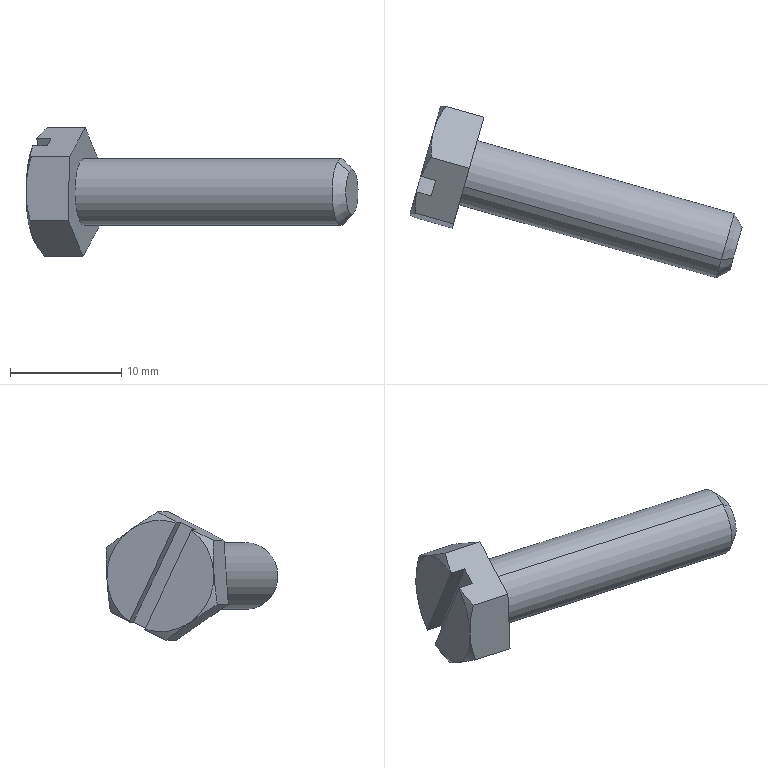Part | SolidWorks | features BaseBody 1 | 1 solid | 23 faces | box 29.808 x 15.418 x 11.521 mm | volume 1021 mm3 | plane 13 | cone 8 | cylinder 2 | commonest cylinder face diameters 6 x2
STEP:
#1=CARTESIAN_POINT('',(393.299,90.116,55.705));
#2=VERTEX_POINT('',#1);
#3=CARTESIAN_POINT('',(392.816,88.42,59.295));
#4=VERTEX_POINT('',#3);
#5=CARTESIAN_POINT('',(393.058,89.268,57.5));
#6=DIRECTION('',(0.9618,-0.2738,0.));
#7=DIRECTION('',(0.1207,0.424,-0.8976));
#8=AXIS2_PLACEMENT_3D('',#5,#6,#7);
#9=CIRCLE('',#8,2.);
#10=EDGE_CURVE('',#2,#4,#9,.T.);
#11=ORIENTED_EDGE('',*,*,#10,.F.);
#12=CARTESIAN_POINT('',(392.458,90.814,54.807));
#13=VERTEX_POINT('',#12);
#14=CARTESIAN_POINT('',(393.299,90.116,55.705));
#15=DIRECTION('',(-0.5947,0.4934,-0.6347));
#16=VECTOR('',#15,1000.);
#17=LINE('',#14,#16);
#18=EDGE_CURVE('',#2,#13,#17,.T.);
#19=ORIENTED_EDGE('',*,*,#18,.T.);
#20=CARTESIAN_POINT('',(391.734,88.27,60.193));
#21=VERTEX_POINT('',#20);
#22=CARTESIAN_POINT('',(392.096,89.542,57.5));
#23=DIRECTION('',(-0.9618,0.2738,0.));
#24=DIRECTION('',(0.1207,0.424,-0.8976));
#25=AXIS2_PLACEMENT_3D('',#22,#23,#24);
#26=CIRCLE('',#25,3.);
#27=EDGE_CURVE('',#21,#13,#26,.T.);
#28=ORIENTED_EDGE('',*,*,#27,.F.);
#29=CARTESIAN_POINT('',(392.816,88.42,59.295));
#30=DIRECTION('',(-0.7654,-0.1062,0.6347));
#31=VECTOR('',#30,1000.);
#32=LINE('',#29,#31);
#33=EDGE_CURVE('',#4,#21,#32,.T.);
#34=ORIENTED_EDGE('',*,*,#33,.F.);
#35=EDGE_LOOP('',(#11,#19,#28,#34));
#36=FACE_OUTER_BOUND('',#35,.T.);
#37=CARTESIAN_POINT('',(393.058,89.268,57.5));
#38=DIRECTION('',(-0.9618,0.2738,0.));
#39=DIRECTION('',(-0.1207,-0.424,0.8976));
#40=AXIS2_PLACEMENT_3D('',#37,#38,#39);
#41=CONICAL_SURFACE('',#40,2.,0.7854);
#42=ADVANCED_FACE('',(#36),#41,.T.);
#43=ORIENTED_EDGE('',*,*,#27,.T.);
#44=CARTESIAN_POINT('',(369.375,97.385,54.807));
#45=VERTEX_POINT('',#44);
#46=CARTESIAN_POINT('',(393.42,90.54,54.807));
#47=DIRECTION('',(-0.9618,0.2738,0.));
#48=VECTOR('',#47,1000.);
#49=LINE('',#46,#48);
#50=EDGE_CURVE('',#13,#45,#49,.T.);
#51=ORIENTED_EDGE('',*,*,#50,.T.);
#52=CARTESIAN_POINT('',(368.651,94.841,60.193));
#53=VERTEX_POINT('',#52);
#54=CARTESIAN_POINT('',(369.013,96.113,57.5));
#55=DIRECTION('',(0.9618,-0.2738,0.));
#56=DIRECTION('',(0.1207,0.424,-0.8976));
#57=AXIS2_PLACEMENT_3D('',#54,#55,#56);
#58=CIRCLE('',#57,3.);
#59=EDGE_CURVE('',#45,#53,#58,.T.);
#60=ORIENTED_EDGE('',*,*,#59,.T.);
#61=CARTESIAN_POINT('',(392.696,87.996,60.193));
#62=DIRECTION('',(-0.9618,0.2738,0.));
#63=VECTOR('',#62,1000.);
#64=LINE('',#61,#63);
#65=EDGE_CURVE('',#21,#53,#64,.T.);
#66=ORIENTED_EDGE('',*,*,#65,.F.);
#67=EDGE_LOOP('',(#43,#51,#60,#66));
#68=FACE_OUTER_BOUND('',#67,.T.);
#69=CARTESIAN_POINT('',(393.058,89.268,57.5));
#70=DIRECTION('',(-0.9618,0.2738,0.));
#71=DIRECTION('',(-0.1207,-0.424,0.8976));
#72=AXIS2_PLACEMENT_3D('',#69,#70,#71);
#73=CYLINDRICAL_SURFACE('',#72,3.);
#74=ADVANCED_FACE('',(#68),#73,.T.);
#75=CARTESIAN_POINT('',(370.432,101.097,60.045));
#76=VERTEX_POINT('',#75);
#77=CARTESIAN_POINT('',(369.119,96.485,63.261));
#78=VERTEX_POINT('',#77);
#79=CARTESIAN_POINT('',(369.119,96.485,63.261));
#80=DIRECTION('',(-0.2274,-0.7988,0.5569));
#81=VECTOR('',#80,1000.);
#82=LINE('',#79,#81);
#83=EDGE_CURVE('',#76,#78,#82,.T.);
#84=ORIENTED_EDGE('',*,*,#83,.T.);
#85=CARTESIAN_POINT('',(367.7,91.501,60.715));
#86=VERTEX_POINT('',#85);
#87=CARTESIAN_POINT('',(367.7,91.501,60.715));
#88=DIRECTION('',(-0.2457,-0.8633,-0.4409));
#89=VECTOR('',#88,1000.);
#90=LINE('',#87,#89);
#91=EDGE_CURVE('',#78,#86,#90,.T.);
#92=ORIENTED_EDGE('',*,*,#91,.T.);
#93=CARTESIAN_POINT('',(367.594,91.129,54.955));
#94=VERTEX_POINT('',#93);
#95=CARTESIAN_POINT('',(367.7,91.501,60.715));
#96=DIRECTION('',(-0.01834,-0.06444,-0.9978));
#97=VECTOR('',#96,1000.);
#98=LINE('',#95,#97);
#99=EDGE_CURVE('',#86,#94,#98,.T.);
#100=ORIENTED_EDGE('',*,*,#99,.T.);
#101=CARTESIAN_POINT('',(368.907,95.741,51.739));
#102=VERTEX_POINT('',#101);
#103=CARTESIAN_POINT('',(368.907,95.741,51.739));
#104=DIRECTION('',(0.2274,0.7988,-0.5569));
#105=VECTOR('',#104,1000.);
#106=LINE('',#103,#105);
#107=EDGE_CURVE('',#94,#102,#106,.T.);
#108=ORIENTED_EDGE('',*,*,#107,.T.);
#109=CARTESIAN_POINT('',(370.326,100.725,54.285));
#110=VERTEX_POINT('',#109);
#111=CARTESIAN_POINT('',(368.907,95.741,51.739));
#112=DIRECTION('',(0.2457,0.8633,0.4409));
#113=VECTOR('',#112,1000.);
#114=LINE('',#111,#113);
#115=EDGE_CURVE('',#102,#110,#114,.T.);
#116=ORIENTED_EDGE('',*,*,#115,.T.);
#117=CARTESIAN_POINT('',(370.326,100.725,54.285));
#118=DIRECTION('',(0.01834,0.06444,0.9978));
#119=VECTOR('',#118,1000.);
#120=LINE('',#117,#119);
#121=EDGE_CURVE('',#110,#76,#120,.T.);
#122=ORIENTED_EDGE('',*,*,#121,.T.);
#123=EDGE_LOOP('',(#84,#92,#100,#108,#116,#122));
#124=FACE_OUTER_BOUND('',#123,.T.);
#125=CARTESIAN_POINT('',(369.013,96.113,57.5));
#126=DIRECTION('',(0.9618,-0.2738,0.));
#127=DIRECTION('',(0.1207,0.424,-0.8976));
#128=AXIS2_PLACEMENT_3D('',#125,#126,#127);
#129=CIRCLE('',#128,3.);
#130=EDGE_CURVE('',#53,#45,#129,.T.);
#131=ORIENTED_EDGE('',*,*,#130,.F.);
#132=ORIENTED_EDGE('',*,*,#59,.F.);
#133=EDGE_LOOP('',(#131,#132));
#134=FACE_BOUND('',#133,.T.);
#135=CARTESIAN_POINT('',(369.119,96.485,63.261));
#136=DIRECTION('',(0.9618,-0.2738,0.));
#137=DIRECTION('',(0.1207,0.424,-0.8976));
#138=AXIS2_PLACEMENT_3D('',#135,#136,#137);
#139=PLANE('',#138);
#140=ADVANCED_FACE('',(#124,#134),#139,.T.);
#141=CARTESIAN_POINT('',(363.8,92.41,57.835));
#142=VERTEX_POINT('',#141);
#143=CARTESIAN_POINT('',(364.374,94.424,61.577));
#144=VERTEX_POINT('',#143);
#145=CARTESIAN_POINT('',(365.166,97.208,57.5));
#146=DIRECTION('',(-0.9618,0.2738,0.));
#147=DIRECTION('',(-0.1207,-0.424,0.8976));
#148=AXIS2_PLACEMENT_3D('',#145,#146,#147);
#149=CIRCLE('',#148,5.);
#150=EDGE_CURVE('',#142,#144,#149,.T.);
#151=ORIENTED_EDGE('',*,*,#150,.T.);
#152=CARTESIAN_POINT('',(365.565,98.61,52.717));
#153=VERTEX_POINT('',#152);
#154=CARTESIAN_POINT('',(365.573,98.637,52.659));
#155=DIRECTION('',(-0.1207,-0.424,0.8976));
#156=VECTOR('',#155,1000.);
#157=LINE('',#154,#156);
#158=EDGE_CURVE('',#153,#144,#157,.T.);
#159=ORIENTED_EDGE('',*,*,#158,.F.);
#160=CARTESIAN_POINT('',(364.404,94.53,53.347));
#161=VERTEX_POINT('',#160);
#162=CARTESIAN_POINT('',(365.166,97.208,57.5));
#163=DIRECTION('',(-0.9618,0.2738,0.));
#164=DIRECTION('',(-0.1207,-0.424,0.8976));
#165=AXIS2_PLACEMENT_3D('',#162,#163,#164);
#166=CIRCLE('',#165,5.);
#167=EDGE_CURVE('',#153,#161,#166,.T.);
#168=ORIENTED_EDGE('',*,*,#167,.T.);
#169=CARTESIAN_POINT('',(365.166,97.208,57.5));
#170=DIRECTION('',(-0.9618,0.2738,0.));
#171=DIRECTION('',(-0.1207,-0.424,0.8976));
#172=AXIS2_PLACEMENT_3D('',#169,#170,#171);
#173=CIRCLE('',#172,5.);
#174=EDGE_CURVE('',#161,#142,#173,.T.);
#175=ORIENTED_EDGE('',*,*,#174,.T.);
#176=EDGE_LOOP('',(#151,#159,#168,#175));
#177=FACE_OUTER_BOUND('',#176,.T.);
#178=CARTESIAN_POINT('',(365.272,97.58,63.261));
#179=DIRECTION('',(0.9618,-0.2738,0.));
#180=DIRECTION('',(0.1207,0.424,-0.8976));
#181=AXIS2_PLACEMENT_3D('',#178,#179,#180);
#182=PLANE('',#181);
#183=ADVANCED_FACE('',(#177),#182,.F.);
#184=CARTESIAN_POINT('',(365.701,97.458,63.261));
#185=VERTEX_POINT('',#184);
#186=CARTESIAN_POINT('',(365.928,99.886,61.653));
#187=VERTEX_POINT('',#186);
#188=CARTESIAN_POINT('',(365.701,97.458,63.261));
#189=CARTESIAN_POINT('',(365.654,98.287,62.735));
#190=CARTESIAN_POINT('',(365.705,99.1,62.201));
#191=CARTESIAN_POINT('',(365.928,99.886,61.653));
#192=B_SPLINE_CURVE_WITH_KNOTS('',3,(#188,#189,#190,#191),.UNSPECIFIED.,.F.,.F.,(4,4),(0.000000238,0.002921),.UNSPECIFIED.);
#193=EDGE_CURVE('',#185,#187,#192,.T.);
#194=ORIENTED_EDGE('',*,*,#193,.F.);
#195=CARTESIAN_POINT('',(369.119,96.485,63.261));
#196=DIRECTION('',(-0.9618,0.2738,0.));
#197=VECTOR('',#196,1000.);
#198=LINE('',#195,#197);
#199=EDGE_CURVE('',#78,#185,#198,.T.);
#200=ORIENTED_EDGE('',*,*,#199,.F.);
#201=ORIENTED_EDGE('',*,*,#83,.F.);
#202=CARTESIAN_POINT('',(367.014,102.07,60.045));
#203=VERTEX_POINT('',#202);
#204=CARTESIAN_POINT('',(370.432,101.097,60.045));
#205=DIRECTION('',(-0.9618,0.2738,0.));
#206=VECTOR('',#205,1000.);
#207=LINE('',#204,#206);
#208=EDGE_CURVE('',#76,#203,#207,.T.);
#209=ORIENTED_EDGE('',*,*,#208,.T.);
#210=CARTESIAN_POINT('',(365.928,99.886,61.653));
#211=CARTESIAN_POINT('',(365.984,100.082,61.516));
#212=CARTESIAN_POINT('',(366.05,100.275,61.379));
#213=CARTESIAN_POINT('',(366.2,100.653,61.108));
#214=CARTESIAN_POINT('',(366.284,100.838,60.974));
#215=CARTESIAN_POINT('',(366.56,101.382,60.572));
#216=CARTESIAN_POINT('',(366.776,101.731,60.308));
#217=CARTESIAN_POINT('',(367.014,102.07,60.045));
#218=B_SPLINE_CURVE_WITH_KNOTS('',3,(#210,#211,#212,#213,#214,#215,#216,#217),.UNSPECIFIED.,.F.,.F.,(4,2,2,4),(0.002921,0.003649,0.004376,0.005831),.UNSPECIFIED.);
#219=EDGE_CURVE('',#187,#203,#218,.T.);
#220=ORIENTED_EDGE('',*,*,#219,.F.);
#221=EDGE_LOOP('',(#194,#200,#201,#209,#220));
#222=FACE_OUTER_BOUND('',#221,.T.);
#223=CARTESIAN_POINT('',(369.119,96.485,63.261));
#224=DIRECTION('',(-0.1525,-0.5356,-0.8306));
#225=DIRECTION('',(0.2274,0.7988,-0.5569));
#226=AXIS2_PLACEMENT_3D('',#223,#224,#225);
#227=PLANE('',#226);
#228=ADVANCED_FACE('',(#222),#227,.F.);
#229=CARTESIAN_POINT('',(364.283,92.473,60.715));
#230=VERTEX_POINT('',#229);
#231=CARTESIAN_POINT('',(364.401,94.387,61.635));
#232=VERTEX_POINT('',#231);
#233=CARTESIAN_POINT('',(364.283,92.473,60.715));
#234=CARTESIAN_POINT('',(364.272,92.795,60.866));
#235=CARTESIAN_POINT('',(364.273,93.119,61.019));
#236=CARTESIAN_POINT('',(364.31,93.758,61.326));
#237=CARTESIAN_POINT('',(364.346,94.075,61.48));
#238=CARTESIAN_POINT('',(364.401,94.387,61.635));
#239=B_SPLINE_CURVE_WITH_KNOTS('',3,(#233,#234,#235,#236,#237,#238),.UNSPECIFIED.,.F.,.F.,(4,2,4),(0.005386,0.006447,0.007508),.UNSPECIFIED.);
#240=EDGE_CURVE('',#230,#232,#239,.T.);
#241=ORIENTED_EDGE('',*,*,#240,.F.);
#242=CARTESIAN_POINT('',(367.7,91.501,60.715));
#243=DIRECTION('',(-0.9618,0.2738,0.));
#244=VECTOR('',#243,1000.);
#245=LINE('',#242,#244);
#246=EDGE_CURVE('',#86,#230,#245,.T.);
#247=ORIENTED_EDGE('',*,*,#246,.F.);
#248=ORIENTED_EDGE('',*,*,#91,.F.);
#249=ORIENTED_EDGE('',*,*,#199,.T.);
#250=CARTESIAN_POINT('',(364.794,95.768,62.341));
#251=VERTEX_POINT('',#250);
#252=CARTESIAN_POINT('',(364.794,95.768,62.341));
#253=CARTESIAN_POINT('',(365.032,96.367,62.655));
#254=CARTESIAN_POINT('',(365.345,96.924,62.961));
#255=CARTESIAN_POINT('',(365.701,97.458,63.261));
#256=B_SPLINE_CURVE_WITH_KNOTS('',3,(#252,#253,#254,#255),.UNSPECIFIED.,.F.,.F.,(4,4),(0.009104,0.01123),.UNSPECIFIED.);
#257=EDGE_CURVE('',#251,#185,#256,.T.);
#258=ORIENTED_EDGE('',*,*,#257,.F.);
#259=CARTESIAN_POINT('',(366.105,95.395,62.341));
#260=VERTEX_POINT('',#259);
#261=CARTESIAN_POINT('',(366.105,95.395,62.341));
#262=DIRECTION('',(-0.9618,0.2738,0.));
#263=VECTOR('',#262,1000.);
#264=LINE('',#261,#263);
#265=EDGE_CURVE('',#260,#251,#264,.T.);
#266=ORIENTED_EDGE('',*,*,#265,.F.);
#267=CARTESIAN_POINT('',(365.712,94.014,61.635));
#268=VERTEX_POINT('',#267);
#269=CARTESIAN_POINT('',(366.105,95.395,62.341));
#270=DIRECTION('',(0.2457,0.8633,0.4409));
#271=VECTOR('',#270,1000.);
#272=LINE('',#269,#271);
#273=EDGE_CURVE('',#268,#260,#272,.T.);
#274=ORIENTED_EDGE('',*,*,#273,.F.);
#275=CARTESIAN_POINT('',(365.712,94.014,61.635));
#276=DIRECTION('',(-0.9618,0.2738,0.));
#277=VECTOR('',#276,1000.);
#278=LINE('',#275,#277);
#279=EDGE_CURVE('',#268,#232,#278,.T.);
#280=ORIENTED_EDGE('',*,*,#279,.T.);
#281=EDGE_LOOP('',(#241,#247,#248,#249,#258,#266,#274,#280));
#282=FACE_OUTER_BOUND('',#281,.T.);
#283=CARTESIAN_POINT('',(367.7,91.501,60.715));
#284=DIRECTION('',(0.1207,0.424,-0.8976));
#285=DIRECTION('',(0.2457,0.8633,0.4409));
#286=AXIS2_PLACEMENT_3D('',#283,#284,#285);
#287=PLANE('',#286);
#288=ADVANCED_FACE('',(#282),#287,.F.);
#289=CARTESIAN_POINT('',(364.177,92.101,54.955));
#290=VERTEX_POINT('',#289);
#291=CARTESIAN_POINT('',(364.177,92.101,54.955));
#292=CARTESIAN_POINT('',(363.932,92.237,55.897));
#293=CARTESIAN_POINT('',(363.782,92.346,56.854));
#294=CARTESIAN_POINT('',(363.8,92.41,57.835));
#295=B_SPLINE_CURVE_WITH_KNOTS('',3,(#291,#292,#293,#294),.UNSPECIFIED.,.F.,.F.,(4,4),(0.000000238,0.002921),.UNSPECIFIED.);
#296=EDGE_CURVE('',#290,#142,#295,.T.);
#297=ORIENTED_EDGE('',*,*,#296,.F.);
#298=CARTESIAN_POINT('',(367.594,91.129,54.955));
#299=DIRECTION('',(-0.9618,0.2738,0.));
#300=VECTOR('',#299,1000.);
#301=LINE('',#298,#300);
#302=EDGE_CURVE('',#94,#290,#301,.T.);
#303=ORIENTED_EDGE('',*,*,#302,.F.);
#304=ORIENTED_EDGE('',*,*,#99,.F.);
#305=ORIENTED_EDGE('',*,*,#246,.T.);
#306=CARTESIAN_POINT('',(363.8,92.41,57.835));
#307=CARTESIAN_POINT('',(363.805,92.425,58.079));
#308=CARTESIAN_POINT('',(363.819,92.438,58.325));
#309=CARTESIAN_POINT('',(363.867,92.459,58.811));
#310=CARTESIAN_POINT('',(363.901,92.466,59.052));
#311=CARTESIAN_POINT('',(364.026,92.48,59.771));
#312=CARTESIAN_POINT('',(364.143,92.48,60.245));
#313=CARTESIAN_POINT('',(364.283,92.473,60.715));
#314=B_SPLINE_CURVE_WITH_KNOTS('',3,(#306,#307,#308,#309,#310,#311,#312,#313),.UNSPECIFIED.,.F.,.F.,(4,2,2,4),(0.002921,0.003649,0.004376,0.005831),.UNSPECIFIED.);
#315=EDGE_CURVE('',#142,#230,#314,.T.);
#316=ORIENTED_EDGE('',*,*,#315,.F.);
#317=EDGE_LOOP('',(#297,#303,#304,#305,#316));
#318=FACE_OUTER_BOUND('',#317,.T.);
#319=CARTESIAN_POINT('',(367.7,91.501,60.715));
#320=DIRECTION('',(0.2732,0.9596,-0.067));
#321=DIRECTION('',(0.01834,0.06444,0.9978));
#322=AXIS2_PLACEMENT_3D('',#319,#320,#321);
#323=PLANE('',#322);
#324=ADVANCED_FACE('',(#318),#323,.F.);
#325=CARTESIAN_POINT('',(365.489,96.714,51.739));
#326=VERTEX_POINT('',#325);
#327=CARTESIAN_POINT('',(365.489,96.714,51.739));
#328=CARTESIAN_POINT('',(365.012,96.034,52.265));
#329=CARTESIAN_POINT('',(364.627,95.315,52.799));
#330=CARTESIAN_POINT('',(364.404,94.53,53.347));
#331=B_SPLINE_CURVE_WITH_KNOTS('',3,(#327,#328,#329,#330),.UNSPECIFIED.,.F.,.F.,(4,4),(0.000000238,0.002921),.UNSPECIFIED.);
#332=EDGE_CURVE('',#326,#161,#331,.T.);
#333=ORIENTED_EDGE('',*,*,#332,.F.);
#334=CARTESIAN_POINT('',(368.907,95.741,51.739));
#335=DIRECTION('',(-0.9618,0.2738,0.));
#336=VECTOR('',#335,1000.);
#337=LINE('',#334,#336);
#338=EDGE_CURVE('',#102,#326,#337,.T.);
#339=ORIENTED_EDGE('',*,*,#338,.F.);
#340=ORIENTED_EDGE('',*,*,#107,.F.);
#341=ORIENTED_EDGE('',*,*,#302,.T.);
#342=CARTESIAN_POINT('',(364.404,94.53,53.347));
#343=CARTESIAN_POINT('',(364.348,94.334,53.484));
#344=CARTESIAN_POINT('',(364.302,94.135,53.621));
#345=CARTESIAN_POINT('',(364.231,93.734,53.892));
#346=CARTESIAN_POINT('',(364.205,93.533,54.026));
#347=CARTESIAN_POINT('',(364.153,92.925,54.428));
#348=CARTESIAN_POINT('',(364.153,92.515,54.692));
#349=CARTESIAN_POINT('',(364.177,92.101,54.955));
#350=B_SPLINE_CURVE_WITH_KNOTS('',3,(#342,#343,#344,#345,#346,#347,#348,#349),.UNSPECIFIED.,.F.,.F.,(4,2,2,4),(0.002921,0.003649,0.004376,0.005831),.UNSPECIFIED.);
#351=EDGE_CURVE('',#161,#290,#350,.T.);
#352=ORIENTED_EDGE('',*,*,#351,.F.);
#353=EDGE_LOOP('',(#333,#339,#340,#341,#352));
#354=FACE_OUTER_BOUND('',#353,.T.);
#355=CARTESIAN_POINT('',(368.907,95.741,51.739));
#356=DIRECTION('',(0.1525,0.5356,0.8306));
#357=DIRECTION('',(-0.2274,-0.7988,0.5569));
#358=AXIS2_PLACEMENT_3D('',#355,#356,#357);
#359=PLANE('',#358);
#360=ADVANCED_FACE('',(#354),#359,.F.);
#361=CARTESIAN_POINT('',(366.908,101.698,54.285));
#362=VERTEX_POINT('',#361);
#363=CARTESIAN_POINT('',(366.001,100.008,53.365));
#364=VERTEX_POINT('',#363);
#365=CARTESIAN_POINT('',(366.908,101.698,54.285));
#366=CARTESIAN_POINT('',(366.552,101.164,53.985));
#367=CARTESIAN_POINT('',(366.239,100.607,53.68));
#368=CARTESIAN_POINT('',(366.001,100.008,53.365));
#369=B_SPLINE_CURVE_WITH_KNOTS('',3,(#365,#366,#367,#368),.UNSPECIFIED.,.F.,.F.,(4,4),(0.0154,0.01752),.UNSPECIFIED.);
#370=EDGE_CURVE('',#362,#364,#369,.T.);
#371=ORIENTED_EDGE('',*,*,#370,.F.);
#372=CARTESIAN_POINT('',(370.326,100.725,54.285));
#373=DIRECTION('',(-0.9618,0.2738,0.));
#374=VECTOR('',#373,1000.);
#375=LINE('',#372,#374);
#376=EDGE_CURVE('',#110,#362,#375,.T.);
#377=ORIENTED_EDGE('',*,*,#376,.F.);
#378=ORIENTED_EDGE('',*,*,#115,.F.);
#379=ORIENTED_EDGE('',*,*,#338,.T.);
#380=CARTESIAN_POINT('',(365.608,98.627,52.659));
#381=VERTEX_POINT('',#380);
#382=CARTESIAN_POINT('',(365.608,98.627,52.659));
#383=CARTESIAN_POINT('',(365.553,98.315,52.504));
#384=CARTESIAN_POINT('',(365.517,97.998,52.35));
#385=CARTESIAN_POINT('',(365.48,97.359,52.043));
#386=CARTESIAN_POINT('',(365.479,97.035,51.89));
#387=CARTESIAN_POINT('',(365.489,96.714,51.739));
#388=B_SPLINE_CURVE_WITH_KNOTS('',3,(#382,#383,#384,#385,#386,#387),.UNSPECIFIED.,.F.,.F.,(4,2,4),(0.01912,0.02018,0.02124),.UNSPECIFIED.);
#389=EDGE_CURVE('',#381,#326,#388,.T.);
#390=ORIENTED_EDGE('',*,*,#389,.F.);
#391=CARTESIAN_POINT('',(366.919,98.254,52.659));
#392=VERTEX_POINT('',#391);
#393=CARTESIAN_POINT('',(366.919,98.254,52.659));
#394=DIRECTION('',(-0.9618,0.2738,0.));
#395=VECTOR('',#394,1000.);
#396=LINE('',#393,#395);
#397=EDGE_CURVE('',#392,#381,#396,.T.);
#398=ORIENTED_EDGE('',*,*,#397,.F.);
#399=CARTESIAN_POINT('',(367.312,99.635,53.365));
#400=VERTEX_POINT('',#399);
#401=CARTESIAN_POINT('',(366.919,98.254,52.659));
#402=DIRECTION('',(-0.2457,-0.8633,-0.4409));
#403=VECTOR('',#402,1000.);
#404=LINE('',#401,#403);
#405=EDGE_CURVE('',#400,#392,#404,.T.);
#406=ORIENTED_EDGE('',*,*,#405,.F.);
#407=CARTESIAN_POINT('',(367.312,99.635,53.365));
#408=DIRECTION('',(-0.9618,0.2738,0.));
#409=VECTOR('',#408,1000.);
#410=LINE('',#407,#409);
#411=EDGE_CURVE('',#400,#364,#410,.T.);
#412=ORIENTED_EDGE('',*,*,#411,.T.);
#413=EDGE_LOOP('',(#371,#377,#378,#379,#390,#398,#406,#412));
#414=FACE_OUTER_BOUND('',#413,.T.);
#415=CARTESIAN_POINT('',(368.907,95.741,51.739));
#416=DIRECTION('',(-0.1207,-0.424,0.8976));
#417=DIRECTION('',(0.9618,-0.2738,0.));
#418=AXIS2_PLACEMENT_3D('',#415,#416,#417);
#419=PLANE('',#418);
#420=ADVANCED_FACE('',(#414),#419,.F.);
#421=CARTESIAN_POINT('',(366.532,102.006,57.165));
#422=VERTEX_POINT('',#421);
#423=CARTESIAN_POINT('',(367.014,102.07,60.045));
#424=CARTESIAN_POINT('',(366.735,102.084,59.103));
#425=CARTESIAN_POINT('',(366.55,102.069,58.146));
#426=CARTESIAN_POINT('',(366.532,102.006,57.165));
#427=B_SPLINE_CURVE_WITH_KNOTS('',3,(#423,#424,#425,#426),.UNSPECIFIED.,.F.,.F.,(4,4),(0.000000238,0.002921),.UNSPECIFIED.);
#428=EDGE_CURVE('',#203,#422,#427,.T.);
#429=ORIENTED_EDGE('',*,*,#428,.F.);
#430=ORIENTED_EDGE('',*,*,#208,.F.);
#431=ORIENTED_EDGE('',*,*,#121,.F.);
#432=ORIENTED_EDGE('',*,*,#376,.T.);
#433=CARTESIAN_POINT('',(366.532,102.006,57.165));
#434=CARTESIAN_POINT('',(366.527,101.99,56.921));
#435=CARTESIAN_POINT('',(366.533,101.971,56.675));
#436=CARTESIAN_POINT('',(366.563,101.929,56.189));
#437=CARTESIAN_POINT('',(366.588,101.905,55.948));
#438=CARTESIAN_POINT('',(366.687,101.827,55.229));
#439=CARTESIAN_POINT('',(366.786,101.765,54.755));
#440=CARTESIAN_POINT('',(366.908,101.698,54.285));
#441=B_SPLINE_CURVE_WITH_KNOTS('',3,(#433,#434,#435,#436,#437,#438,#439,#440),.UNSPECIFIED.,.F.,.F.,(4,2,2,4),(0.002921,0.003649,0.004376,0.005831),.UNSPECIFIED.);
#442=EDGE_CURVE('',#422,#362,#441,.T.);
#443=ORIENTED_EDGE('',*,*,#442,.F.);
#444=EDGE_LOOP('',(#429,#430,#431,#432,#443));
#445=FACE_OUTER_BOUND('',#444,.T.);
#446=CARTESIAN_POINT('',(370.326,100.725,54.285));
#447=DIRECTION('',(-0.2732,-0.9596,0.067));
#448=DIRECTION('',(-0.01834,-0.06444,-0.9978));
#449=AXIS2_PLACEMENT_3D('',#446,#447,#448);
#450=PLANE('',#449);
#451=ADVANCED_FACE('',(#445),#450,.F.);
#452=CARTESIAN_POINT('',(365.958,99.991,53.423));
#453=VERTEX_POINT('',#452);
#454=CARTESIAN_POINT('',(365.166,97.208,57.5));
#455=DIRECTION('',(-0.9618,0.2738,0.));
#456=DIRECTION('',(-0.1207,-0.424,0.8976));
#457=AXIS2_PLACEMENT_3D('',#454,#455,#456);
#458=CIRCLE('',#457,5.);
#459=EDGE_CURVE('',#422,#453,#458,.T.);
#460=ORIENTED_EDGE('',*,*,#459,.T.);
#461=CARTESIAN_POINT('',(364.767,95.806,62.283));
#462=VERTEX_POINT('',#461);
#463=CARTESIAN_POINT('',(365.966,100.019,53.365));
#464=DIRECTION('',(0.1207,0.424,-0.8976));
#465=VECTOR('',#464,1000.);
#466=LINE('',#463,#465);
#467=EDGE_CURVE('',#462,#453,#466,.T.);
#468=ORIENTED_EDGE('',*,*,#467,.F.);
#469=CARTESIAN_POINT('',(365.166,97.208,57.5));
#470=DIRECTION('',(-0.9618,0.2738,0.));
#471=DIRECTION('',(-0.1207,-0.424,0.8976));
#472=AXIS2_PLACEMENT_3D('',#469,#470,#471);
#473=CIRCLE('',#472,5.);
#474=EDGE_CURVE('',#462,#187,#473,.T.);
#475=ORIENTED_EDGE('',*,*,#474,.T.);
#476=CARTESIAN_POINT('',(365.166,97.208,57.5));
#477=DIRECTION('',(-0.9618,0.2738,0.));
#478=DIRECTION('',(-0.1207,-0.424,0.8976));
#479=AXIS2_PLACEMENT_3D('',#476,#477,#478);
#480=CIRCLE('',#479,5.);
#481=EDGE_CURVE('',#187,#422,#480,.T.);
#482=ORIENTED_EDGE('',*,*,#481,.T.);
#483=EDGE_LOOP('',(#460,#468,#475,#482));
#484=FACE_OUTER_BOUND('',#483,.T.);
#485=CARTESIAN_POINT('',(365.272,97.58,63.261));
#486=DIRECTION('',(0.9618,-0.2738,0.));
#487=DIRECTION('',(0.1207,0.424,-0.8976));
#488=AXIS2_PLACEMENT_3D('',#485,#486,#487);
#489=PLANE('',#488);
#490=ADVANCED_FACE('',(#484),#489,.F.);
#491=CARTESIAN_POINT('',(364.401,94.387,61.635));
#492=CARTESIAN_POINT('',(364.392,94.4,61.616));
#493=CARTESIAN_POINT('',(364.383,94.412,61.597));
#494=CARTESIAN_POINT('',(364.374,94.424,61.577));
#495=B_SPLINE_CURVE_WITH_KNOTS('',3,(#491,#492,#493,#494),.UNSPECIFIED.,.F.,.F.,(4,4),(0.006986,0.00706),.UNSPECIFIED.);
#496=EDGE_CURVE('',#232,#144,#495,.T.);
#497=ORIENTED_EDGE('',*,*,#496,.F.);
#498=ORIENTED_EDGE('',*,*,#279,.F.);
#499=CARTESIAN_POINT('',(366.919,98.254,52.659));
#500=DIRECTION('',(-0.1207,-0.424,0.8976));
#501=VECTOR('',#500,1000.);
#502=LINE('',#499,#501);
#503=EDGE_CURVE('',#392,#268,#502,.T.);
#504=ORIENTED_EDGE('',*,*,#503,.F.);
#505=ORIENTED_EDGE('',*,*,#397,.T.);
#506=CARTESIAN_POINT('',(365.565,98.61,52.717));
#507=CARTESIAN_POINT('',(365.579,98.616,52.698));
#508=CARTESIAN_POINT('',(365.594,98.621,52.679));
#509=CARTESIAN_POINT('',(365.608,98.627,52.659));
#510=B_SPLINE_CURVE_WITH_KNOTS('',3,(#506,#507,#508,#509),.UNSPECIFIED.,.F.,.F.,(4,4),(0.01814,0.01822),.UNSPECIFIED.);
#511=EDGE_CURVE('',#153,#381,#510,.T.);
#512=ORIENTED_EDGE('',*,*,#511,.F.);
#513=ORIENTED_EDGE('',*,*,#158,.T.);
#514=EDGE_LOOP('',(#497,#498,#504,#505,#512,#513));
#515=FACE_OUTER_BOUND('',#514,.T.);
#516=CARTESIAN_POINT('',(366.919,98.254,52.659));
#517=DIRECTION('',(-0.2457,-0.8633,-0.4409));
#518=DIRECTION('',(-0.9618,0.2738,0.));
#519=AXIS2_PLACEMENT_3D('',#516,#517,#518);
#520=PLANE('',#519);
#521=ADVANCED_FACE('',(#515),#520,.F.);
#522=CARTESIAN_POINT('',(366.001,100.008,53.365));
#523=CARTESIAN_POINT('',(365.987,100.003,53.384));
#524=CARTESIAN_POINT('',(365.973,99.997,53.403));
#525=CARTESIAN_POINT('',(365.958,99.991,53.423));
#526=B_SPLINE_CURVE_WITH_KNOTS('',3,(#522,#523,#524,#525),.UNSPECIFIED.,.F.,.F.,(4,4),(0.006986,0.00706),.UNSPECIFIED.);
#527=EDGE_CURVE('',#364,#453,#526,.T.);
#528=ORIENTED_EDGE('',*,*,#527,.F.);
#529=ORIENTED_EDGE('',*,*,#411,.F.);
#530=CARTESIAN_POINT('',(367.312,99.635,53.365));
#531=DIRECTION('',(0.1207,0.424,-0.8976));
#532=VECTOR('',#531,1000.);
#533=LINE('',#530,#532);
#534=EDGE_CURVE('',#260,#400,#533,.T.);
#535=ORIENTED_EDGE('',*,*,#534,.F.);
#536=ORIENTED_EDGE('',*,*,#265,.T.);
#537=CARTESIAN_POINT('',(364.767,95.806,62.283));
#538=CARTESIAN_POINT('',(364.776,95.793,62.302));
#539=CARTESIAN_POINT('',(364.785,95.781,62.321));
#540=CARTESIAN_POINT('',(364.794,95.768,62.341));
#541=B_SPLINE_CURVE_WITH_KNOTS('',3,(#537,#538,#539,#540),.UNSPECIFIED.,.F.,.F.,(4,4),(0.01814,0.01822),.UNSPECIFIED.);
#542=EDGE_CURVE('',#462,#251,#541,.T.);
#543=ORIENTED_EDGE('',*,*,#542,.F.);
#544=ORIENTED_EDGE('',*,*,#467,.T.);
#545=EDGE_LOOP('',(#528,#529,#535,#536,#543,#544));
#546=FACE_OUTER_BOUND('',#545,.T.);
#547=CARTESIAN_POINT('',(367.312,99.635,53.365));
#548=DIRECTION('',(0.2457,0.8633,0.4409));
#549=DIRECTION('',(0.9618,-0.2738,0.));
#550=AXIS2_PLACEMENT_3D('',#547,#548,#549);
#551=PLANE('',#550);
#552=ADVANCED_FACE('',(#546),#551,.F.);
#553=ORIENTED_EDGE('',*,*,#273,.T.);
#554=ORIENTED_EDGE('',*,*,#534,.T.);
#555=ORIENTED_EDGE('',*,*,#405,.T.);
#556=ORIENTED_EDGE('',*,*,#503,.T.);
#557=EDGE_LOOP('',(#553,#554,#555,#556));
#558=FACE_OUTER_BOUND('',#557,.T.);
#559=CARTESIAN_POINT('',(365.712,94.014,61.635));
#560=DIRECTION('',(-0.9618,0.2738,0.));
#561=DIRECTION('',(-0.1207,-0.424,0.8976));
#562=AXIS2_PLACEMENT_3D('',#559,#560,#561);
#563=PLANE('',#562);
#564=ADVANCED_FACE('',(#558),#563,.T.);
#565=ORIENTED_EDGE('',*,*,#193,.T.);
#566=ORIENTED_EDGE('',*,*,#474,.F.);
#567=ORIENTED_EDGE('',*,*,#542,.T.);
#568=ORIENTED_EDGE('',*,*,#257,.T.);
#569=EDGE_LOOP('',(#565,#566,#567,#568));
#570=FACE_OUTER_BOUND('',#569,.T.);
#571=CARTESIAN_POINT('',(365.166,97.208,57.5));
#572=DIRECTION('',(0.9618,-0.2738,0.));
#573=DIRECTION('',(-0.1207,-0.424,0.8976));
#574=AXIS2_PLACEMENT_3D('',#571,#572,#573);
#575=CONICAL_SURFACE('',#574,5.,1.047);
#576=ADVANCED_FACE('',(#570),#575,.T.);
#577=ORIENTED_EDGE('',*,*,#527,.T.);
#578=ORIENTED_EDGE('',*,*,#459,.F.);
#579=ORIENTED_EDGE('',*,*,#442,.T.);
#580=ORIENTED_EDGE('',*,*,#370,.T.);
#581=EDGE_LOOP('',(#577,#578,#579,#580));
#582=FACE_OUTER_BOUND('',#581,.T.);
#583=CARTESIAN_POINT('',(365.166,97.208,57.5));
#584=DIRECTION('',(0.9618,-0.2738,0.));
#585=DIRECTION('',(-0.1207,-0.424,0.8976));
#586=AXIS2_PLACEMENT_3D('',#583,#584,#585);
#587=CONICAL_SURFACE('',#586,5.,1.047);
#588=ADVANCED_FACE('',(#582),#587,.T.);
#589=ORIENTED_EDGE('',*,*,#332,.T.);
#590=ORIENTED_EDGE('',*,*,#167,.F.);
#591=ORIENTED_EDGE('',*,*,#511,.T.);
#592=ORIENTED_EDGE('',*,*,#389,.T.);
#593=EDGE_LOOP('',(#589,#590,#591,#592));
#594=FACE_OUTER_BOUND('',#593,.T.);
#595=CARTESIAN_POINT('',(365.166,97.208,57.5));
#596=DIRECTION('',(0.9618,-0.2738,0.));
#597=DIRECTION('',(-0.1207,-0.424,0.8976));
#598=AXIS2_PLACEMENT_3D('',#595,#596,#597);
#599=CONICAL_SURFACE('',#598,5.,1.047);
#600=ADVANCED_FACE('',(#594),#599,.T.);
#601=ORIENTED_EDGE('',*,*,#496,.T.);
#602=ORIENTED_EDGE('',*,*,#150,.F.);
#603=ORIENTED_EDGE('',*,*,#315,.T.);
#604=ORIENTED_EDGE('',*,*,#240,.T.);
#605=EDGE_LOOP('',(#601,#602,#603,#604));
#606=FACE_OUTER_BOUND('',#605,.T.);
#607=CARTESIAN_POINT('',(365.166,97.208,57.5));
#608=DIRECTION('',(0.9618,-0.2738,0.));
#609=DIRECTION('',(-0.1207,-0.424,0.8976));
#610=AXIS2_PLACEMENT_3D('',#607,#608,#609);
#611=CONICAL_SURFACE('',#610,5.,1.047);
#612=ADVANCED_FACE('',(#606),#611,.T.);
#613=ORIENTED_EDGE('',*,*,#428,.T.);
#614=ORIENTED_EDGE('',*,*,#481,.F.);
#615=ORIENTED_EDGE('',*,*,#219,.T.);
#616=EDGE_LOOP('',(#613,#614,#615));
#617=FACE_OUTER_BOUND('',#616,.T.);
#618=CARTESIAN_POINT('',(365.166,97.208,57.5));
#619=DIRECTION('',(0.9618,-0.2738,0.));
#620=DIRECTION('',(-0.1207,-0.424,0.8976));
#621=AXIS2_PLACEMENT_3D('',#618,#619,#620);
#622=CONICAL_SURFACE('',#621,5.,1.047);
#623=ADVANCED_FACE('',(#617),#622,.T.);
#624=ORIENTED_EDGE('',*,*,#296,.T.);
#625=ORIENTED_EDGE('',*,*,#174,.F.);
#626=ORIENTED_EDGE('',*,*,#351,.T.);
#627=EDGE_LOOP('',(#624,#625,#626));
#628=FACE_OUTER_BOUND('',#627,.T.);
#629=CARTESIAN_POINT('',(365.166,97.208,57.5));
#630=DIRECTION('',(0.9618,-0.2738,0.));
#631=DIRECTION('',(-0.1207,-0.424,0.8976));
#632=AXIS2_PLACEMENT_3D('',#629,#630,#631);
#633=CONICAL_SURFACE('',#632,5.,1.047);
#634=ADVANCED_FACE('',(#628),#633,.T.);
#635=ORIENTED_EDGE('',*,*,#50,.F.);
#636=CARTESIAN_POINT('',(392.096,89.542,57.5));
#637=DIRECTION('',(-0.9618,0.2738,0.));
#638=DIRECTION('',(0.1207,0.424,-0.8976));
#639=AXIS2_PLACEMENT_3D('',#636,#637,#638);
#640=CIRCLE('',#639,3.);
#641=EDGE_CURVE('',#13,#21,#640,.T.);
#642=ORIENTED_EDGE('',*,*,#641,.T.);
#643=ORIENTED_EDGE('',*,*,#65,.T.);
#644=ORIENTED_EDGE('',*,*,#130,.T.);
#645=EDGE_LOOP('',(#635,#642,#643,#644));
#646=FACE_OUTER_BOUND('',#645,.T.);
#647=CARTESIAN_POINT('',(393.058,89.268,57.5));
#648=DIRECTION('',(-0.9618,0.2738,0.));
#649=DIRECTION('',(-0.1207,-0.424,0.8976));
#650=AXIS2_PLACEMENT_3D('',#647,#648,#649);
#651=CYLINDRICAL_SURFACE('',#650,3.);
#652=ADVANCED_FACE('',(#646),#651,.T.);
#653=CARTESIAN_POINT('',(393.058,89.268,57.5));
#654=DIRECTION('',(0.9618,-0.2738,0.));
#655=DIRECTION('',(0.1207,0.424,-0.8976));
#656=AXIS2_PLACEMENT_3D('',#653,#654,#655);
#657=CIRCLE('',#656,2.);
#658=EDGE_CURVE('',#4,#2,#657,.T.);
#659=ORIENTED_EDGE('',*,*,#658,.T.);
#660=ORIENTED_EDGE('',*,*,#10,.T.);
#661=EDGE_LOOP('',(#659,#660));
#662=FACE_OUTER_BOUND('',#661,.T.);
#663=CARTESIAN_POINT('',(393.058,89.268,57.5));
#664=DIRECTION('',(0.9618,-0.2738,0.));
#665=DIRECTION('',(0.1207,0.424,-0.8976));
#666=AXIS2_PLACEMENT_3D('',#663,#664,#665);
#667=PLANE('',#666);
#668=ADVANCED_FACE('',(#662),#667,.T.);
#669=ORIENTED_EDGE('',*,*,#18,.F.);
#670=ORIENTED_EDGE('',*,*,#658,.F.);
#671=ORIENTED_EDGE('',*,*,#33,.T.);
#672=ORIENTED_EDGE('',*,*,#641,.F.);
#673=EDGE_LOOP('',(#669,#670,#671,#672));
#674=FACE_OUTER_BOUND('',#673,.T.);
#675=CARTESIAN_POINT('',(393.058,89.268,57.5));
#676=DIRECTION('',(-0.9618,0.2738,0.));
#677=DIRECTION('',(-0.1207,-0.424,0.8976));
#678=AXIS2_PLACEMENT_3D('',#675,#676,#677);
#679=CONICAL_SURFACE('',#678,2.,0.7854);
#680=ADVANCED_FACE('',(#674),#679,.T.);
#681=CLOSED_SHELL('',(#42,#74,#140,#183,#228,#288,#324,#360,#420,#451,#490,#521,#552,#564,#576,#588,#600,#612,#623,#634,#652,#668,#680));
#682=MANIFOLD_SOLID_BREP('',#681);
#683=CARTESIAN_POINT('',(0.,0.,0.));
#684=DIRECTION('',(0.,0.,1.));
#685=DIRECTION('',(1.,0.,0.));
#686=AXIS2_PLACEMENT_3D('',#683,#684,#685);
#687=(LENGTH_UNIT()NAMED_UNIT(*)SI_UNIT(.MILLI.,.METRE.));
#688=UNCERTAINTY_MEASURE_WITH_UNIT(LENGTH_MEASURE(0.00001),#687,'','');
#689=(NAMED_UNIT(*)PLANE_ANGLE_UNIT()SI_UNIT($,.RADIAN.));
#690=(NAMED_UNIT(*)SI_UNIT($,.STERADIAN.)SOLID_ANGLE_UNIT());
#691=(GEOMETRIC_REPRESENTATION_CONTEXT(3)GLOBAL_UNCERTAINTY_ASSIGNED_CONTEXT((#688))GLOBAL_UNIT_ASSIGNED_CONTEXT((#687,#689,#690))REPRESENTATION_CONTEXT('',''));
#692=ADVANCED_BREP_SHAPE_REPRESENTATION('',(#682,#686),#691);